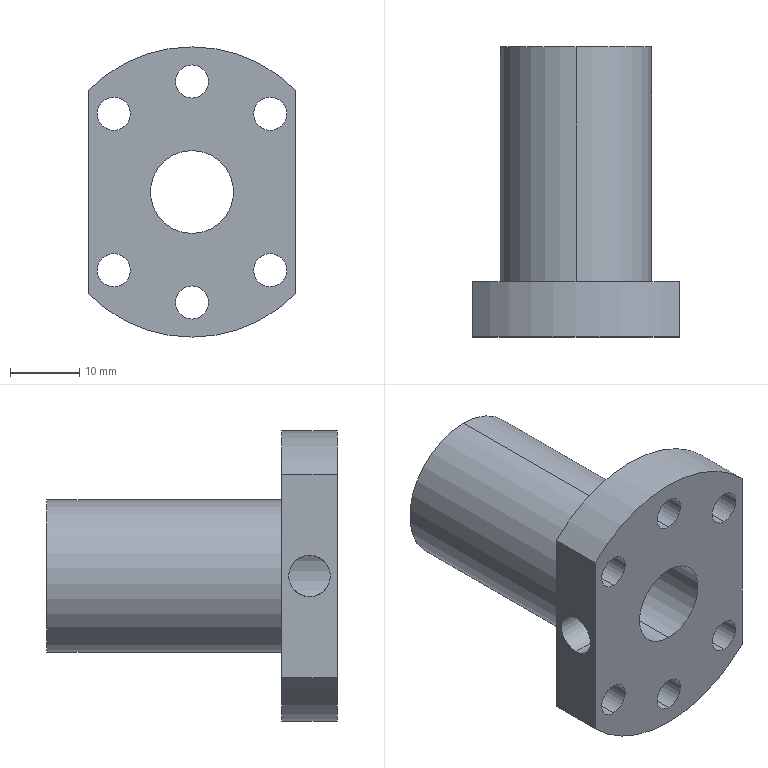Part | SolidWorks | features BaseBody 1 | 1 solid | 26 faces | box 30 x 42 x 42 mm | volume 16187 mm3 | cylinder 21 | plane 5 | commonest cylinder face diameters 4.8 x12 42 x3 6 x2 12 x2 22 x2
STEP:
#1=CARTESIAN_POINT('',(0.,42.,-11.));
#2=VERTEX_POINT('',#1);
#3=CARTESIAN_POINT('',(0.,42.,11.));
#4=VERTEX_POINT('',#3);
#5=CARTESIAN_POINT('',(0.,42.,0.));
#6=DIRECTION('',(0.,-1.,0.));
#7=DIRECTION('',(0.,0.,-1.));
#8=AXIS2_PLACEMENT_3D('',#5,#6,#7);
#9=CIRCLE('',#8,11.);
#10=EDGE_CURVE('',#2,#4,#9,.T.);
#11=ORIENTED_EDGE('',*,*,#10,.T.);
#12=CARTESIAN_POINT('',(0.,8.,11.));
#13=VERTEX_POINT('',#12);
#14=CARTESIAN_POINT('',(0.,42.,11.));
#15=DIRECTION('',(0.,-1.,0.));
#16=VECTOR('',#15,1000.);
#17=LINE('',#14,#16);
#18=EDGE_CURVE('',#4,#13,#17,.T.);
#19=ORIENTED_EDGE('',*,*,#18,.T.);
#20=CARTESIAN_POINT('',(0.,8.,-11.));
#21=VERTEX_POINT('',#20);
#22=CARTESIAN_POINT('',(0.,8.,0.));
#23=DIRECTION('',(0.,1.,0.));
#24=DIRECTION('',(0.,0.,-1.));
#25=AXIS2_PLACEMENT_3D('',#22,#23,#24);
#26=CIRCLE('',#25,11.);
#27=EDGE_CURVE('',#13,#21,#26,.T.);
#28=ORIENTED_EDGE('',*,*,#27,.T.);
#29=CARTESIAN_POINT('',(0.,42.,-11.));
#30=DIRECTION('',(0.,-1.,0.));
#31=VECTOR('',#30,1000.);
#32=LINE('',#29,#31);
#33=EDGE_CURVE('',#2,#21,#32,.T.);
#34=ORIENTED_EDGE('',*,*,#33,.F.);
#35=EDGE_LOOP('',(#11,#19,#28,#34));
#36=FACE_OUTER_BOUND('',#35,.T.);
#37=CARTESIAN_POINT('',(0.,42.,0.));
#38=DIRECTION('',(0.,-1.,0.));
#39=DIRECTION('',(0.,0.,-1.));
#40=AXIS2_PLACEMENT_3D('',#37,#38,#39);
#41=CYLINDRICAL_SURFACE('',#40,11.);
#42=ADVANCED_FACE('',(#36),#41,.T.);
#43=CARTESIAN_POINT('',(-11.314,8.,-8.914));
#44=VERTEX_POINT('',#43);
#45=CARTESIAN_POINT('',(-11.314,8.,-13.714));
#46=VERTEX_POINT('',#45);
#47=CARTESIAN_POINT('',(-11.314,8.,-11.314));
#48=DIRECTION('',(0.,-1.,0.));
#49=DIRECTION('',(0.,0.,-1.));
#50=AXIS2_PLACEMENT_3D('',#47,#48,#49);
#51=CIRCLE('',#50,2.4);
#52=EDGE_CURVE('',#44,#46,#51,.T.);
#53=ORIENTED_EDGE('',*,*,#52,.F.);
#54=CARTESIAN_POINT('',(-11.314,0.,-8.914));
#55=VERTEX_POINT('',#54);
#56=CARTESIAN_POINT('',(-11.314,8.,-8.914));
#57=DIRECTION('',(0.,-1.,0.));
#58=VECTOR('',#57,1000.);
#59=LINE('',#56,#58);
#60=EDGE_CURVE('',#44,#55,#59,.T.);
#61=ORIENTED_EDGE('',*,*,#60,.T.);
#62=CARTESIAN_POINT('',(-11.314,0.,-13.714));
#63=VERTEX_POINT('',#62);
#64=CARTESIAN_POINT('',(-11.314,0.,-11.314));
#65=DIRECTION('',(0.,1.,0.));
#66=DIRECTION('',(0.,0.,-1.));
#67=AXIS2_PLACEMENT_3D('',#64,#65,#66);
#68=CIRCLE('',#67,2.4);
#69=EDGE_CURVE('',#63,#55,#68,.T.);
#70=ORIENTED_EDGE('',*,*,#69,.F.);
#71=CARTESIAN_POINT('',(-11.314,8.,-13.714));
#72=DIRECTION('',(0.,-1.,0.));
#73=VECTOR('',#72,1000.);
#74=LINE('',#71,#73);
#75=EDGE_CURVE('',#46,#63,#74,.T.);
#76=ORIENTED_EDGE('',*,*,#75,.F.);
#77=EDGE_LOOP('',(#53,#61,#70,#76));
#78=FACE_OUTER_BOUND('',#77,.T.);
#79=CARTESIAN_POINT('',(-11.314,8.,-11.314));
#80=DIRECTION('',(0.,-1.,0.));
#81=DIRECTION('',(0.,0.,-1.));
#82=AXIS2_PLACEMENT_3D('',#79,#80,#81);
#83=CYLINDRICAL_SURFACE('',#82,2.4);
#84=ADVANCED_FACE('',(#78),#83,.F.);
#85=CARTESIAN_POINT('',(11.314,8.,13.714));
#86=VERTEX_POINT('',#85);
#87=CARTESIAN_POINT('',(11.314,8.,8.914));
#88=VERTEX_POINT('',#87);
#89=CARTESIAN_POINT('',(11.314,8.,11.314));
#90=DIRECTION('',(0.,-1.,0.));
#91=DIRECTION('',(0.,0.,-1.));
#92=AXIS2_PLACEMENT_3D('',#89,#90,#91);
#93=CIRCLE('',#92,2.4);
#94=EDGE_CURVE('',#86,#88,#93,.T.);
#95=ORIENTED_EDGE('',*,*,#94,.F.);
#96=CARTESIAN_POINT('',(11.314,0.,13.714));
#97=VERTEX_POINT('',#96);
#98=CARTESIAN_POINT('',(11.314,8.,13.714));
#99=DIRECTION('',(0.,-1.,0.));
#100=VECTOR('',#99,1000.);
#101=LINE('',#98,#100);
#102=EDGE_CURVE('',#86,#97,#101,.T.);
#103=ORIENTED_EDGE('',*,*,#102,.T.);
#104=CARTESIAN_POINT('',(11.314,0.,8.914));
#105=VERTEX_POINT('',#104);
#106=CARTESIAN_POINT('',(11.314,0.,11.314));
#107=DIRECTION('',(0.,1.,0.));
#108=DIRECTION('',(0.,0.,-1.));
#109=AXIS2_PLACEMENT_3D('',#106,#107,#108);
#110=CIRCLE('',#109,2.4);
#111=EDGE_CURVE('',#105,#97,#110,.T.);
#112=ORIENTED_EDGE('',*,*,#111,.F.);
#113=CARTESIAN_POINT('',(11.314,8.,8.914));
#114=DIRECTION('',(0.,-1.,0.));
#115=VECTOR('',#114,1000.);
#116=LINE('',#113,#115);
#117=EDGE_CURVE('',#88,#105,#116,.T.);
#118=ORIENTED_EDGE('',*,*,#117,.F.);
#119=EDGE_LOOP('',(#95,#103,#112,#118));
#120=FACE_OUTER_BOUND('',#119,.T.);
#121=CARTESIAN_POINT('',(11.314,8.,11.314));
#122=DIRECTION('',(0.,-1.,0.));
#123=DIRECTION('',(0.,0.,-1.));
#124=AXIS2_PLACEMENT_3D('',#121,#122,#123);
#125=CYLINDRICAL_SURFACE('',#124,2.4);
#126=ADVANCED_FACE('',(#120),#125,.F.);
#127=CARTESIAN_POINT('',(-11.314,8.,13.714));
#128=VERTEX_POINT('',#127);
#129=CARTESIAN_POINT('',(-11.314,8.,8.914));
#130=VERTEX_POINT('',#129);
#131=CARTESIAN_POINT('',(-11.314,8.,11.314));
#132=DIRECTION('',(0.,-1.,0.));
#133=DIRECTION('',(0.,0.,-1.));
#134=AXIS2_PLACEMENT_3D('',#131,#132,#133);
#135=CIRCLE('',#134,2.4);
#136=EDGE_CURVE('',#128,#130,#135,.T.);
#137=ORIENTED_EDGE('',*,*,#136,.F.);
#138=CARTESIAN_POINT('',(-11.314,0.,13.714));
#139=VERTEX_POINT('',#138);
#140=CARTESIAN_POINT('',(-11.314,8.,13.714));
#141=DIRECTION('',(0.,-1.,0.));
#142=VECTOR('',#141,1000.);
#143=LINE('',#140,#142);
#144=EDGE_CURVE('',#128,#139,#143,.T.);
#145=ORIENTED_EDGE('',*,*,#144,.T.);
#146=CARTESIAN_POINT('',(-11.314,0.,8.914));
#147=VERTEX_POINT('',#146);
#148=CARTESIAN_POINT('',(-11.314,0.,11.314));
#149=DIRECTION('',(0.,1.,0.));
#150=DIRECTION('',(0.,0.,-1.));
#151=AXIS2_PLACEMENT_3D('',#148,#149,#150);
#152=CIRCLE('',#151,2.4);
#153=EDGE_CURVE('',#147,#139,#152,.T.);
#154=ORIENTED_EDGE('',*,*,#153,.F.);
#155=CARTESIAN_POINT('',(-11.314,8.,8.914));
#156=DIRECTION('',(0.,-1.,0.));
#157=VECTOR('',#156,1000.);
#158=LINE('',#155,#157);
#159=EDGE_CURVE('',#130,#147,#158,.T.);
#160=ORIENTED_EDGE('',*,*,#159,.F.);
#161=EDGE_LOOP('',(#137,#145,#154,#160));
#162=FACE_OUTER_BOUND('',#161,.T.);
#163=CARTESIAN_POINT('',(-11.314,8.,11.314));
#164=DIRECTION('',(0.,-1.,0.));
#165=DIRECTION('',(0.,0.,-1.));
#166=AXIS2_PLACEMENT_3D('',#163,#164,#165);
#167=CYLINDRICAL_SURFACE('',#166,2.4);
#168=ADVANCED_FACE('',(#162),#167,.F.);
#169=CARTESIAN_POINT('',(0.,8.,18.4));
#170=VERTEX_POINT('',#169);
#171=CARTESIAN_POINT('',(0.,8.,13.6));
#172=VERTEX_POINT('',#171);
#173=CARTESIAN_POINT('',(0.,8.,16.));
#174=DIRECTION('',(0.,-1.,0.));
#175=DIRECTION('',(0.,0.,-1.));
#176=AXIS2_PLACEMENT_3D('',#173,#174,#175);
#177=CIRCLE('',#176,2.4);
#178=EDGE_CURVE('',#170,#172,#177,.T.);
#179=ORIENTED_EDGE('',*,*,#178,.F.);
#180=CARTESIAN_POINT('',(0.,0.,18.4));
#181=VERTEX_POINT('',#180);
#182=CARTESIAN_POINT('',(0.,8.,18.4));
#183=DIRECTION('',(0.,-1.,0.));
#184=VECTOR('',#183,1000.);
#185=LINE('',#182,#184);
#186=EDGE_CURVE('',#170,#181,#185,.T.);
#187=ORIENTED_EDGE('',*,*,#186,.T.);
#188=CARTESIAN_POINT('',(0.,0.,13.6));
#189=VERTEX_POINT('',#188);
#190=CARTESIAN_POINT('',(0.,0.,16.));
#191=DIRECTION('',(0.,1.,0.));
#192=DIRECTION('',(0.,0.,-1.));
#193=AXIS2_PLACEMENT_3D('',#190,#191,#192);
#194=CIRCLE('',#193,2.4);
#195=EDGE_CURVE('',#189,#181,#194,.T.);
#196=ORIENTED_EDGE('',*,*,#195,.F.);
#197=CARTESIAN_POINT('',(0.,8.,13.6));
#198=DIRECTION('',(0.,-1.,0.));
#199=VECTOR('',#198,1000.);
#200=LINE('',#197,#199);
#201=EDGE_CURVE('',#172,#189,#200,.T.);
#202=ORIENTED_EDGE('',*,*,#201,.F.);
#203=EDGE_LOOP('',(#179,#187,#196,#202));
#204=FACE_OUTER_BOUND('',#203,.T.);
#205=CARTESIAN_POINT('',(0.,8.,16.));
#206=DIRECTION('',(0.,-1.,0.));
#207=DIRECTION('',(0.,0.,-1.));
#208=AXIS2_PLACEMENT_3D('',#205,#206,#207);
#209=CYLINDRICAL_SURFACE('',#208,2.4);
#210=ADVANCED_FACE('',(#204),#209,.F.);
#211=CARTESIAN_POINT('',(0.,8.,-21.));
#212=VERTEX_POINT('',#211);
#213=CARTESIAN_POINT('',(-15.,8.,-14.697));
#214=VERTEX_POINT('',#213);
#215=CARTESIAN_POINT('',(0.,8.,0.));
#216=DIRECTION('',(0.,1.,0.));
#217=DIRECTION('',(0.,0.,-1.));
#218=AXIS2_PLACEMENT_3D('',#215,#216,#217);
#219=CIRCLE('',#218,21.);
#220=EDGE_CURVE('',#212,#214,#219,.T.);
#221=ORIENTED_EDGE('',*,*,#220,.F.);
#222=CARTESIAN_POINT('',(0.,0.,-21.));
#223=VERTEX_POINT('',#222);
#224=CARTESIAN_POINT('',(0.,8.,-21.));
#225=DIRECTION('',(0.,-1.,0.));
#226=VECTOR('',#225,1000.);
#227=LINE('',#224,#226);
#228=EDGE_CURVE('',#212,#223,#227,.T.);
#229=ORIENTED_EDGE('',*,*,#228,.T.);
#230=CARTESIAN_POINT('',(-15.,0.,-14.697));
#231=VERTEX_POINT('',#230);
#232=CARTESIAN_POINT('',(0.,0.,0.));
#233=DIRECTION('',(0.,1.,0.));
#234=DIRECTION('',(0.,0.,-1.));
#235=AXIS2_PLACEMENT_3D('',#232,#233,#234);
#236=CIRCLE('',#235,21.);
#237=EDGE_CURVE('',#223,#231,#236,.T.);
#238=ORIENTED_EDGE('',*,*,#237,.T.);
#239=CARTESIAN_POINT('',(-15.,8.,-14.697));
#240=DIRECTION('',(0.,1.,0.));
#241=VECTOR('',#240,1000.);
#242=LINE('',#239,#241);
#243=EDGE_CURVE('',#231,#214,#242,.T.);
#244=ORIENTED_EDGE('',*,*,#243,.T.);
#245=EDGE_LOOP('',(#221,#229,#238,#244));
#246=FACE_OUTER_BOUND('',#245,.T.);
#247=CARTESIAN_POINT('',(0.,8.,0.));
#248=DIRECTION('',(0.,-1.,0.));
#249=DIRECTION('',(0.,0.,-1.));
#250=AXIS2_PLACEMENT_3D('',#247,#248,#249);
#251=CYLINDRICAL_SURFACE('',#250,21.);
#252=ADVANCED_FACE('',(#246),#251,.T.);
#253=CARTESIAN_POINT('',(11.314,8.,-8.914));
#254=VERTEX_POINT('',#253);
#255=CARTESIAN_POINT('',(11.314,8.,-13.714));
#256=VERTEX_POINT('',#255);
#257=CARTESIAN_POINT('',(11.314,8.,-11.314));
#258=DIRECTION('',(0.,-1.,0.));
#259=DIRECTION('',(0.,0.,-1.));
#260=AXIS2_PLACEMENT_3D('',#257,#258,#259);
#261=CIRCLE('',#260,2.4);
#262=EDGE_CURVE('',#254,#256,#261,.T.);
#263=ORIENTED_EDGE('',*,*,#262,.F.);
#264=CARTESIAN_POINT('',(11.314,0.,-8.914));
#265=VERTEX_POINT('',#264);
#266=CARTESIAN_POINT('',(11.314,8.,-8.914));
#267=DIRECTION('',(0.,-1.,0.));
#268=VECTOR('',#267,1000.);
#269=LINE('',#266,#268);
#270=EDGE_CURVE('',#254,#265,#269,.T.);
#271=ORIENTED_EDGE('',*,*,#270,.T.);
#272=CARTESIAN_POINT('',(11.314,0.,-13.714));
#273=VERTEX_POINT('',#272);
#274=CARTESIAN_POINT('',(11.314,0.,-11.314));
#275=DIRECTION('',(0.,1.,0.));
#276=DIRECTION('',(0.,0.,-1.));
#277=AXIS2_PLACEMENT_3D('',#274,#275,#276);
#278=CIRCLE('',#277,2.4);
#279=EDGE_CURVE('',#273,#265,#278,.T.);
#280=ORIENTED_EDGE('',*,*,#279,.F.);
#281=CARTESIAN_POINT('',(11.314,8.,-13.714));
#282=DIRECTION('',(0.,-1.,0.));
#283=VECTOR('',#282,1000.);
#284=LINE('',#281,#283);
#285=EDGE_CURVE('',#256,#273,#284,.T.);
#286=ORIENTED_EDGE('',*,*,#285,.F.);
#287=EDGE_LOOP('',(#263,#271,#280,#286));
#288=FACE_OUTER_BOUND('',#287,.T.);
#289=CARTESIAN_POINT('',(11.314,8.,-11.314));
#290=DIRECTION('',(0.,-1.,0.));
#291=DIRECTION('',(0.,0.,-1.));
#292=AXIS2_PLACEMENT_3D('',#289,#290,#291);
#293=CYLINDRICAL_SURFACE('',#292,2.4);
#294=ADVANCED_FACE('',(#288),#293,.F.);
#295=CARTESIAN_POINT('',(0.,8.,-13.6));
#296=VERTEX_POINT('',#295);
#297=CARTESIAN_POINT('',(0.,8.,-18.4));
#298=VERTEX_POINT('',#297);
#299=CARTESIAN_POINT('',(0.,8.,-16.));
#300=DIRECTION('',(0.,-1.,0.));
#301=DIRECTION('',(0.,0.,-1.));
#302=AXIS2_PLACEMENT_3D('',#299,#300,#301);
#303=CIRCLE('',#302,2.4);
#304=EDGE_CURVE('',#296,#298,#303,.T.);
#305=ORIENTED_EDGE('',*,*,#304,.F.);
#306=CARTESIAN_POINT('',(0.,0.,-13.6));
#307=VERTEX_POINT('',#306);
#308=CARTESIAN_POINT('',(0.,8.,-13.6));
#309=DIRECTION('',(0.,-1.,0.));
#310=VECTOR('',#309,1000.);
#311=LINE('',#308,#310);
#312=EDGE_CURVE('',#296,#307,#311,.T.);
#313=ORIENTED_EDGE('',*,*,#312,.T.);
#314=CARTESIAN_POINT('',(0.,0.,-18.4));
#315=VERTEX_POINT('',#314);
#316=CARTESIAN_POINT('',(0.,0.,-16.));
#317=DIRECTION('',(0.,1.,0.));
#318=DIRECTION('',(0.,0.,-1.));
#319=AXIS2_PLACEMENT_3D('',#316,#317,#318);
#320=CIRCLE('',#319,2.4);
#321=EDGE_CURVE('',#315,#307,#320,.T.);
#322=ORIENTED_EDGE('',*,*,#321,.F.);
#323=CARTESIAN_POINT('',(0.,8.,-18.4));
#324=DIRECTION('',(0.,-1.,0.));
#325=VECTOR('',#324,1000.);
#326=LINE('',#323,#325);
#327=EDGE_CURVE('',#298,#315,#326,.T.);
#328=ORIENTED_EDGE('',*,*,#327,.F.);
#329=EDGE_LOOP('',(#305,#313,#322,#328));
#330=FACE_OUTER_BOUND('',#329,.T.);
#331=CARTESIAN_POINT('',(0.,8.,-16.));
#332=DIRECTION('',(0.,-1.,0.));
#333=DIRECTION('',(0.,0.,-1.));
#334=AXIS2_PLACEMENT_3D('',#331,#332,#333);
#335=CYLINDRICAL_SURFACE('',#334,2.4);
#336=ADVANCED_FACE('',(#330),#335,.F.);
#337=CARTESIAN_POINT('',(-5.196,4.,3.));
#338=VERTEX_POINT('',#337);
#339=CARTESIAN_POINT('',(-5.196,4.,-3.));
#340=VERTEX_POINT('',#339);
#341=CARTESIAN_POINT('',(-5.196,4.,3.));
#342=CARTESIAN_POINT('',(-5.196,3.798,3.));
#343=CARTESIAN_POINT('',(-5.208,3.6,2.98));
#344=CARTESIAN_POINT('',(-5.252,3.213,2.902));
#345=CARTESIAN_POINT('',(-5.285,3.021,2.843));
#346=CARTESIAN_POINT('',(-5.363,2.66,2.691));
#347=CARTESIAN_POINT('',(-5.409,2.489,2.599));
#348=CARTESIAN_POINT('',(-5.508,2.166,2.382));
#349=CARTESIAN_POINT('',(-5.56,2.016,2.259));
#350=CARTESIAN_POINT('',(-5.663,1.744,1.987));
#351=CARTESIAN_POINT('',(-5.714,1.62,1.837));
#352=CARTESIAN_POINT('',(-5.808,1.403,1.514));
#353=CARTESIAN_POINT('',(-5.851,1.31,1.343));
#354=CARTESIAN_POINT('',(-5.922,1.159,0.9829));
#355=CARTESIAN_POINT('',(-5.951,1.099,0.7906));
#356=CARTESIAN_POINT('',(-5.99,1.02,0.4015));
#357=CARTESIAN_POINT('',(-6.,1.,0.2044));
#358=CARTESIAN_POINT('',(-6.,0.9997,-0.1952));
#359=CARTESIAN_POINT('',(-5.99,1.02,-0.3971));
#360=CARTESIAN_POINT('',(-5.952,1.098,-0.7856));
#361=CARTESIAN_POINT('',(-5.923,1.156,-0.9764));
#362=CARTESIAN_POINT('',(-5.851,1.309,-1.341));
#363=CARTESIAN_POINT('',(-5.809,1.402,-1.512));
#364=CARTESIAN_POINT('',(-5.715,1.618,-1.835));
#365=CARTESIAN_POINT('',(-5.664,1.743,-1.986));
#366=CARTESIAN_POINT('',(-5.561,2.016,-2.258));
#367=CARTESIAN_POINT('',(-5.509,2.164,-2.381));
#368=CARTESIAN_POINT('',(-5.41,2.488,-2.598));
#369=CARTESIAN_POINT('',(-5.364,2.659,-2.691));
#370=CARTESIAN_POINT('',(-5.285,3.018,-2.841));
#371=CARTESIAN_POINT('',(-5.253,3.207,-2.9));
#372=CARTESIAN_POINT('',(-5.208,3.599,-2.98));
#373=CARTESIAN_POINT('',(-5.196,3.798,-3.));
#374=CARTESIAN_POINT('',(-5.196,4.,-3.));
#375=B_SPLINE_CURVE_WITH_KNOTS('',3,(#341,#342,#343,#344,#345,#346,#347,#348,#349,#350,#351,#352,#353,#354,#355,#356,#357,#358,#359,#360,#361,#362,#363,#364,#365,#366,#367,#368,#369,#370,#371,#372,#373,#374),.UNSPECIFIED.,.F.,.F.,(4,2,2,2,2,2,2,2,2,2,2,2,2,2,2,2,4),(0.,0.000596,0.001192,0.001788,0.002384,0.00298,0.003576,0.004172,0.004768,0.005364,0.00596,0.006556,0.007152,0.007748,0.008344,0.00894,0.009537),.UNSPECIFIED.);
#376=EDGE_CURVE('',#338,#340,#375,.T.);
#377=ORIENTED_EDGE('',*,*,#376,.F.);
#378=CARTESIAN_POINT('',(-5.196,4.,-3.));
#379=CARTESIAN_POINT('',(-5.196,4.202,-3.));
#380=CARTESIAN_POINT('',(-5.208,4.4,-2.98));
#381=CARTESIAN_POINT('',(-5.252,4.787,-2.902));
#382=CARTESIAN_POINT('',(-5.285,4.979,-2.843));
#383=CARTESIAN_POINT('',(-5.363,5.34,-2.691));
#384=CARTESIAN_POINT('',(-5.409,5.511,-2.599));
#385=CARTESIAN_POINT('',(-5.508,5.834,-2.382));
#386=CARTESIAN_POINT('',(-5.56,5.984,-2.259));
#387=CARTESIAN_POINT('',(-5.663,6.256,-1.987));
#388=CARTESIAN_POINT('',(-5.714,6.38,-1.837));
#389=CARTESIAN_POINT('',(-5.808,6.597,-1.514));
#390=CARTESIAN_POINT('',(-5.851,6.69,-1.343));
#391=CARTESIAN_POINT('',(-5.922,6.841,-0.9829));
#392=CARTESIAN_POINT('',(-5.951,6.901,-0.7906));
#393=CARTESIAN_POINT('',(-5.99,6.98,-0.4015));
#394=CARTESIAN_POINT('',(-6.,7.,-0.2044));
#395=CARTESIAN_POINT('',(-6.,7.,0.1952));
#396=CARTESIAN_POINT('',(-5.99,6.98,0.3971));
#397=CARTESIAN_POINT('',(-5.952,6.902,0.7856));
#398=CARTESIAN_POINT('',(-5.923,6.844,0.9764));
#399=CARTESIAN_POINT('',(-5.851,6.691,1.341));
#400=CARTESIAN_POINT('',(-5.809,6.598,1.512));
#401=CARTESIAN_POINT('',(-5.715,6.382,1.835));
#402=CARTESIAN_POINT('',(-5.664,6.257,1.986));
#403=CARTESIAN_POINT('',(-5.561,5.984,2.258));
#404=CARTESIAN_POINT('',(-5.509,5.836,2.381));
#405=CARTESIAN_POINT('',(-5.41,5.512,2.598));
#406=CARTESIAN_POINT('',(-5.364,5.341,2.691));
#407=CARTESIAN_POINT('',(-5.285,4.982,2.841));
#408=CARTESIAN_POINT('',(-5.253,4.793,2.9));
#409=CARTESIAN_POINT('',(-5.208,4.401,2.98));
#410=CARTESIAN_POINT('',(-5.196,4.202,3.));
#411=CARTESIAN_POINT('',(-5.196,4.,3.));
#412=B_SPLINE_CURVE_WITH_KNOTS('',3,(#378,#379,#380,#381,#382,#383,#384,#385,#386,#387,#388,#389,#390,#391,#392,#393,#394,#395,#396,#397,#398,#399,#400,#401,#402,#403,#404,#405,#406,#407,#408,#409,#410,#411),.UNSPECIFIED.,.F.,.F.,(4,2,2,2,2,2,2,2,2,2,2,2,2,2,2,2,4),(0.009537,0.01013,0.01073,0.01132,0.01192,0.01251,0.01311,0.01371,0.0143,0.0149,0.01549,0.01609,0.01668,0.01728,0.01788,0.01847,0.01907),.UNSPECIFIED.);
#413=EDGE_CURVE('',#340,#338,#412,.T.);
#414=ORIENTED_EDGE('',*,*,#413,.F.);
#415=EDGE_LOOP('',(#377,#414));
#416=FACE_BOUND('',#415,.T.);
#417=CARTESIAN_POINT('',(0.,42.,6.));
#418=VERTEX_POINT('',#417);
#419=CARTESIAN_POINT('',(0.,42.,-6.));
#420=VERTEX_POINT('',#419);
#421=CARTESIAN_POINT('',(0.,42.,0.));
#422=DIRECTION('',(0.,-1.,0.));
#423=DIRECTION('',(0.,0.,-1.));
#424=AXIS2_PLACEMENT_3D('',#421,#422,#423);
#425=CIRCLE('',#424,6.);
#426=EDGE_CURVE('',#418,#420,#425,.T.);
#427=ORIENTED_EDGE('',*,*,#426,.F.);
#428=CARTESIAN_POINT('',(0.,0.,6.));
#429=VERTEX_POINT('',#428);
#430=CARTESIAN_POINT('',(0.,42.,6.));
#431=DIRECTION('',(0.,-1.,0.));
#432=VECTOR('',#431,1000.);
#433=LINE('',#430,#432);
#434=EDGE_CURVE('',#418,#429,#433,.T.);
#435=ORIENTED_EDGE('',*,*,#434,.T.);
#436=CARTESIAN_POINT('',(0.,0.,-6.));
#437=VERTEX_POINT('',#436);
#438=CARTESIAN_POINT('',(0.,0.,0.));
#439=DIRECTION('',(0.,1.,0.));
#440=DIRECTION('',(0.,0.,-1.));
#441=AXIS2_PLACEMENT_3D('',#438,#439,#440);
#442=CIRCLE('',#441,6.);
#443=EDGE_CURVE('',#437,#429,#442,.T.);
#444=ORIENTED_EDGE('',*,*,#443,.F.);
#445=CARTESIAN_POINT('',(0.,42.,-6.));
#446=DIRECTION('',(0.,-1.,0.));
#447=VECTOR('',#446,1000.);
#448=LINE('',#445,#447);
#449=EDGE_CURVE('',#420,#437,#448,.T.);
#450=ORIENTED_EDGE('',*,*,#449,.F.);
#451=EDGE_LOOP('',(#427,#435,#444,#450));
#452=FACE_OUTER_BOUND('',#451,.T.);
#453=CARTESIAN_POINT('',(0.,42.,0.));
#454=DIRECTION('',(0.,-1.,0.));
#455=DIRECTION('',(0.,0.,-1.));
#456=AXIS2_PLACEMENT_3D('',#453,#454,#455);
#457=CYLINDRICAL_SURFACE('',#456,6.);
#458=ADVANCED_FACE('',(#416,#452),#457,.F.);
#459=ORIENTED_EDGE('',*,*,#376,.T.);
#460=CARTESIAN_POINT('',(-15.,4.,-3.));
#461=VERTEX_POINT('',#460);
#462=CARTESIAN_POINT('',(5.,4.,-3.));
#463=DIRECTION('',(-1.,0.,0.));
#464=VECTOR('',#463,1000.);
#465=LINE('',#462,#464);
#466=EDGE_CURVE('',#340,#461,#465,.T.);
#467=ORIENTED_EDGE('',*,*,#466,.T.);
#468=CARTESIAN_POINT('',(-15.,4.,3.));
#469=VERTEX_POINT('',#468);
#470=CARTESIAN_POINT('',(-15.,4.,0.));
#471=DIRECTION('',(-1.,0.,0.));
#472=DIRECTION('',(0.,0.,1.));
#473=AXIS2_PLACEMENT_3D('',#470,#471,#472);
#474=CIRCLE('',#473,3.);
#475=EDGE_CURVE('',#461,#469,#474,.T.);
#476=ORIENTED_EDGE('',*,*,#475,.T.);
#477=CARTESIAN_POINT('',(5.,4.,3.));
#478=DIRECTION('',(-1.,0.,0.));
#479=VECTOR('',#478,1000.);
#480=LINE('',#477,#479);
#481=EDGE_CURVE('',#338,#469,#480,.T.);
#482=ORIENTED_EDGE('',*,*,#481,.F.);
#483=EDGE_LOOP('',(#459,#467,#476,#482));
#484=FACE_OUTER_BOUND('',#483,.T.);
#485=CARTESIAN_POINT('',(5.,4.,0.));
#486=DIRECTION('',(-1.,0.,0.));
#487=DIRECTION('',(0.,0.,1.));
#488=AXIS2_PLACEMENT_3D('',#485,#486,#487);
#489=CYLINDRICAL_SURFACE('',#488,3.);
#490=ADVANCED_FACE('',(#484),#489,.F.);
#491=ORIENTED_EDGE('',*,*,#18,.F.);
#492=CARTESIAN_POINT('',(0.,42.,0.));
#493=DIRECTION('',(0.,-1.,0.));
#494=DIRECTION('',(0.,0.,-1.));
#495=AXIS2_PLACEMENT_3D('',#492,#493,#494);
#496=CIRCLE('',#495,11.);
#497=EDGE_CURVE('',#4,#2,#496,.T.);
#498=ORIENTED_EDGE('',*,*,#497,.T.);
#499=ORIENTED_EDGE('',*,*,#33,.T.);
#500=CARTESIAN_POINT('',(0.,8.,0.));
#501=DIRECTION('',(0.,1.,0.));
#502=DIRECTION('',(0.,0.,-1.));
#503=AXIS2_PLACEMENT_3D('',#500,#501,#502);
#504=CIRCLE('',#503,11.);
#505=EDGE_CURVE('',#21,#13,#504,.T.);
#506=ORIENTED_EDGE('',*,*,#505,.T.);
#507=EDGE_LOOP('',(#491,#498,#499,#506));
#508=FACE_OUTER_BOUND('',#507,.T.);
#509=CARTESIAN_POINT('',(0.,42.,0.));
#510=DIRECTION('',(0.,-1.,0.));
#511=DIRECTION('',(0.,0.,-1.));
#512=AXIS2_PLACEMENT_3D('',#509,#510,#511);
#513=CYLINDRICAL_SURFACE('',#512,11.);
#514=ADVANCED_FACE('',(#508),#513,.T.);
#515=CARTESIAN_POINT('',(-11.314,8.,-11.314));
#516=DIRECTION('',(0.,-1.,0.));
#517=DIRECTION('',(0.,0.,-1.));
#518=AXIS2_PLACEMENT_3D('',#515,#516,#517);
#519=CIRCLE('',#518,2.4);
#520=EDGE_CURVE('',#46,#44,#519,.T.);
#521=ORIENTED_EDGE('',*,*,#520,.T.);
#522=ORIENTED_EDGE('',*,*,#52,.T.);
#523=EDGE_LOOP('',(#521,#522));
#524=FACE_BOUND('',#523,.T.);
#525=CARTESIAN_POINT('',(11.314,8.,11.314));
#526=DIRECTION('',(0.,-1.,0.));
#527=DIRECTION('',(0.,0.,-1.));
#528=AXIS2_PLACEMENT_3D('',#525,#526,#527);
#529=CIRCLE('',#528,2.4);
#530=EDGE_CURVE('',#88,#86,#529,.T.);
#531=ORIENTED_EDGE('',*,*,#530,.T.);
#532=ORIENTED_EDGE('',*,*,#94,.T.);
#533=EDGE_LOOP('',(#531,#532));
#534=FACE_BOUND('',#533,.T.);
#535=CARTESIAN_POINT('',(-11.314,8.,11.314));
#536=DIRECTION('',(0.,-1.,0.));
#537=DIRECTION('',(0.,0.,-1.));
#538=AXIS2_PLACEMENT_3D('',#535,#536,#537);
#539=CIRCLE('',#538,2.4);
#540=EDGE_CURVE('',#130,#128,#539,.T.);
#541=ORIENTED_EDGE('',*,*,#540,.T.);
#542=ORIENTED_EDGE('',*,*,#136,.T.);
#543=EDGE_LOOP('',(#541,#542));
#544=FACE_BOUND('',#543,.T.);
#545=CARTESIAN_POINT('',(0.,8.,16.));
#546=DIRECTION('',(0.,-1.,0.));
#547=DIRECTION('',(0.,0.,-1.));
#548=AXIS2_PLACEMENT_3D('',#545,#546,#547);
#549=CIRCLE('',#548,2.4);
#550=EDGE_CURVE('',#172,#170,#549,.T.);
#551=ORIENTED_EDGE('',*,*,#550,.T.);
#552=ORIENTED_EDGE('',*,*,#178,.T.);
#553=EDGE_LOOP('',(#551,#552));
#554=FACE_BOUND('',#553,.T.);
#555=ORIENTED_EDGE('',*,*,#505,.F.);
#556=ORIENTED_EDGE('',*,*,#27,.F.);
#557=EDGE_LOOP('',(#555,#556));
#558=FACE_BOUND('',#557,.T.);
#559=CARTESIAN_POINT('',(-15.,8.,14.697));
#560=VERTEX_POINT('',#559);
#561=CARTESIAN_POINT('',(-15.,8.,0.));
#562=DIRECTION('',(0.,0.,1.));
#563=VECTOR('',#562,1000.);
#564=LINE('',#561,#563);
#565=EDGE_CURVE('',#214,#560,#564,.T.);
#566=ORIENTED_EDGE('',*,*,#565,.T.);
#567=CARTESIAN_POINT('',(15.,8.,14.697));
#568=VERTEX_POINT('',#567);
#569=CARTESIAN_POINT('',(0.,8.,0.));
#570=DIRECTION('',(0.,1.,0.));
#571=DIRECTION('',(0.,0.,-1.));
#572=AXIS2_PLACEMENT_3D('',#569,#570,#571);
#573=CIRCLE('',#572,21.);
#574=EDGE_CURVE('',#560,#568,#573,.T.);
#575=ORIENTED_EDGE('',*,*,#574,.T.);
#576=CARTESIAN_POINT('',(15.,8.,-14.697));
#577=VERTEX_POINT('',#576);
#578=CARTESIAN_POINT('',(15.,8.,0.));
#579=DIRECTION('',(0.,0.,-1.));
#580=VECTOR('',#579,1000.);
#581=LINE('',#578,#580);
#582=EDGE_CURVE('',#568,#577,#581,.T.);
#583=ORIENTED_EDGE('',*,*,#582,.T.);
#584=CARTESIAN_POINT('',(0.,8.,0.));
#585=DIRECTION('',(0.,1.,0.));
#586=DIRECTION('',(0.,0.,-1.));
#587=AXIS2_PLACEMENT_3D('',#584,#585,#586);
#588=CIRCLE('',#587,21.);
#589=EDGE_CURVE('',#577,#212,#588,.T.);
#590=ORIENTED_EDGE('',*,*,#589,.T.);
#591=ORIENTED_EDGE('',*,*,#220,.T.);
#592=EDGE_LOOP('',(#566,#575,#583,#590,#591));
#593=FACE_OUTER_BOUND('',#592,.T.);
#594=CARTESIAN_POINT('',(11.314,8.,-11.314));
#595=DIRECTION('',(0.,-1.,0.));
#596=DIRECTION('',(0.,0.,-1.));
#597=AXIS2_PLACEMENT_3D('',#594,#595,#596);
#598=CIRCLE('',#597,2.4);
#599=EDGE_CURVE('',#256,#254,#598,.T.);
#600=ORIENTED_EDGE('',*,*,#599,.T.);
#601=ORIENTED_EDGE('',*,*,#262,.T.);
#602=EDGE_LOOP('',(#600,#601));
#603=FACE_BOUND('',#602,.T.);
#604=CARTESIAN_POINT('',(0.,8.,-16.));
#605=DIRECTION('',(0.,-1.,0.));
#606=DIRECTION('',(0.,0.,-1.));
#607=AXIS2_PLACEMENT_3D('',#604,#605,#606);
#608=CIRCLE('',#607,2.4);
#609=EDGE_CURVE('',#298,#296,#608,.T.);
#610=ORIENTED_EDGE('',*,*,#609,.T.);
#611=ORIENTED_EDGE('',*,*,#304,.T.);
#612=EDGE_LOOP('',(#610,#611));
#613=FACE_BOUND('',#612,.T.);
#614=CARTESIAN_POINT('',(0.,8.,0.));
#615=DIRECTION('',(0.,1.,0.));
#616=DIRECTION('',(0.,0.,1.));
#617=AXIS2_PLACEMENT_3D('',#614,#615,#616);
#618=PLANE('',#617);
#619=ADVANCED_FACE('',(#524,#534,#544,#554,#558,#593,#603,#613),#618,.T.);
#620=ORIENTED_EDGE('',*,*,#10,.F.);
#621=ORIENTED_EDGE('',*,*,#497,.F.);
#622=EDGE_LOOP('',(#620,#621));
#623=FACE_OUTER_BOUND('',#622,.T.);
#624=CARTESIAN_POINT('',(0.,42.,0.));
#625=DIRECTION('',(0.,-1.,0.));
#626=DIRECTION('',(0.,0.,-1.));
#627=AXIS2_PLACEMENT_3D('',#624,#625,#626);
#628=CIRCLE('',#627,6.);
#629=EDGE_CURVE('',#420,#418,#628,.T.);
#630=ORIENTED_EDGE('',*,*,#629,.T.);
#631=ORIENTED_EDGE('',*,*,#426,.T.);
#632=EDGE_LOOP('',(#630,#631));
#633=FACE_BOUND('',#632,.T.);
#634=CARTESIAN_POINT('',(0.,42.,0.));
#635=DIRECTION('',(0.,1.,0.));
#636=DIRECTION('',(0.,0.,1.));
#637=AXIS2_PLACEMENT_3D('',#634,#635,#636);
#638=PLANE('',#637);
#639=ADVANCED_FACE('',(#623,#633),#638,.T.);
#640=ORIENTED_EDGE('',*,*,#60,.F.);
#641=ORIENTED_EDGE('',*,*,#520,.F.);
#642=ORIENTED_EDGE('',*,*,#75,.T.);
#643=CARTESIAN_POINT('',(-11.314,0.,-11.314));
#644=DIRECTION('',(0.,1.,0.));
#645=DIRECTION('',(0.,0.,-1.));
#646=AXIS2_PLACEMENT_3D('',#643,#644,#645);
#647=CIRCLE('',#646,2.4);
#648=EDGE_CURVE('',#55,#63,#647,.T.);
#649=ORIENTED_EDGE('',*,*,#648,.F.);
#650=EDGE_LOOP('',(#640,#641,#642,#649));
#651=FACE_OUTER_BOUND('',#650,.T.);
#652=CARTESIAN_POINT('',(-11.314,8.,-11.314));
#653=DIRECTION('',(0.,-1.,0.));
#654=DIRECTION('',(0.,0.,-1.));
#655=AXIS2_PLACEMENT_3D('',#652,#653,#654);
#656=CYLINDRICAL_SURFACE('',#655,2.4);
#657=ADVANCED_FACE('',(#651),#656,.F.);
#658=ORIENTED_EDGE('',*,*,#102,.F.);
#659=ORIENTED_EDGE('',*,*,#530,.F.);
#660=ORIENTED_EDGE('',*,*,#117,.T.);
#661=CARTESIAN_POINT('',(11.314,0.,11.314));
#662=DIRECTION('',(0.,1.,0.));
#663=DIRECTION('',(0.,0.,-1.));
#664=AXIS2_PLACEMENT_3D('',#661,#662,#663);
#665=CIRCLE('',#664,2.4);
#666=EDGE_CURVE('',#97,#105,#665,.T.);
#667=ORIENTED_EDGE('',*,*,#666,.F.);
#668=EDGE_LOOP('',(#658,#659,#660,#667));
#669=FACE_OUTER_BOUND('',#668,.T.);
#670=CARTESIAN_POINT('',(11.314,8.,11.314));
#671=DIRECTION('',(0.,-1.,0.));
#672=DIRECTION('',(0.,0.,-1.));
#673=AXIS2_PLACEMENT_3D('',#670,#671,#672);
#674=CYLINDRICAL_SURFACE('',#673,2.4);
#675=ADVANCED_FACE('',(#669),#674,.F.);
#676=ORIENTED_EDGE('',*,*,#144,.F.);
#677=ORIENTED_EDGE('',*,*,#540,.F.);
#678=ORIENTED_EDGE('',*,*,#159,.T.);
#679=CARTESIAN_POINT('',(-11.314,0.,11.314));
#680=DIRECTION('',(0.,1.,0.));
#681=DIRECTION('',(0.,0.,-1.));
#682=AXIS2_PLACEMENT_3D('',#679,#680,#681);
#683=CIRCLE('',#682,2.4);
#684=EDGE_CURVE('',#139,#147,#683,.T.);
#685=ORIENTED_EDGE('',*,*,#684,.F.);
#686=EDGE_LOOP('',(#676,#677,#678,#685));
#687=FACE_OUTER_BOUND('',#686,.T.);
#688=CARTESIAN_POINT('',(-11.314,8.,11.314));
#689=DIRECTION('',(0.,-1.,0.));
#690=DIRECTION('',(0.,0.,-1.));
#691=AXIS2_PLACEMENT_3D('',#688,#689,#690);
#692=CYLINDRICAL_SURFACE('',#691,2.4);
#693=ADVANCED_FACE('',(#687),#692,.F.);
#694=ORIENTED_EDGE('',*,*,#186,.F.);
#695=ORIENTED_EDGE('',*,*,#550,.F.);
#696=ORIENTED_EDGE('',*,*,#201,.T.);
#697=CARTESIAN_POINT('',(0.,0.,16.));
#698=DIRECTION('',(0.,1.,0.));
#699=DIRECTION('',(0.,0.,-1.));
#700=AXIS2_PLACEMENT_3D('',#697,#698,#699);
#701=CIRCLE('',#700,2.4);
#702=EDGE_CURVE('',#181,#189,#701,.T.);
#703=ORIENTED_EDGE('',*,*,#702,.F.);
#704=EDGE_LOOP('',(#694,#695,#696,#703));
#705=FACE_OUTER_BOUND('',#704,.T.);
#706=CARTESIAN_POINT('',(0.,8.,16.));
#707=DIRECTION('',(0.,-1.,0.));
#708=DIRECTION('',(0.,0.,-1.));
#709=AXIS2_PLACEMENT_3D('',#706,#707,#708);
#710=CYLINDRICAL_SURFACE('',#709,2.4);
#711=ADVANCED_FACE('',(#705),#710,.F.);
#712=ORIENTED_EDGE('',*,*,#574,.F.);
#713=CARTESIAN_POINT('',(-15.,0.,14.697));
#714=VERTEX_POINT('',#713);
#715=CARTESIAN_POINT('',(-15.,8.,14.697));
#716=DIRECTION('',(0.,-1.,0.));
#717=VECTOR('',#716,1000.);
#718=LINE('',#715,#717);
#719=EDGE_CURVE('',#560,#714,#718,.T.);
#720=ORIENTED_EDGE('',*,*,#719,.T.);
#721=CARTESIAN_POINT('',(15.,0.,14.697));
#722=VERTEX_POINT('',#721);
#723=CARTESIAN_POINT('',(0.,0.,0.));
#724=DIRECTION('',(0.,1.,0.));
#725=DIRECTION('',(0.,0.,-1.));
#726=AXIS2_PLACEMENT_3D('',#723,#724,#725);
#727=CIRCLE('',#726,21.);
#728=EDGE_CURVE('',#714,#722,#727,.T.);
#729=ORIENTED_EDGE('',*,*,#728,.T.);
#730=CARTESIAN_POINT('',(15.,8.,14.697));
#731=DIRECTION('',(0.,1.,0.));
#732=VECTOR('',#731,1000.);
#733=LINE('',#730,#732);
#734=EDGE_CURVE('',#722,#568,#733,.T.);
#735=ORIENTED_EDGE('',*,*,#734,.T.);
#736=EDGE_LOOP('',(#712,#720,#729,#735));
#737=FACE_OUTER_BOUND('',#736,.T.);
#738=CARTESIAN_POINT('',(0.,8.,0.));
#739=DIRECTION('',(0.,-1.,0.));
#740=DIRECTION('',(0.,0.,-1.));
#741=AXIS2_PLACEMENT_3D('',#738,#739,#740);
#742=CYLINDRICAL_SURFACE('',#741,21.);
#743=ADVANCED_FACE('',(#737),#742,.T.);
#744=ORIENTED_EDGE('',*,*,#719,.F.);
#745=ORIENTED_EDGE('',*,*,#565,.F.);
#746=ORIENTED_EDGE('',*,*,#243,.F.);
#747=CARTESIAN_POINT('',(-15.,0.,0.));
#748=DIRECTION('',(0.,0.,-1.));
#749=VECTOR('',#748,1000.);
#750=LINE('',#747,#749);
#751=EDGE_CURVE('',#714,#231,#750,.T.);
#752=ORIENTED_EDGE('',*,*,#751,.F.);
#753=EDGE_LOOP('',(#744,#745,#746,#752));
#754=FACE_OUTER_BOUND('',#753,.T.);
#755=CARTESIAN_POINT('',(-15.,4.,0.));
#756=DIRECTION('',(-1.,0.,0.));
#757=DIRECTION('',(0.,0.,1.));
#758=AXIS2_PLACEMENT_3D('',#755,#756,#757);
#759=CIRCLE('',#758,3.);
#760=EDGE_CURVE('',#469,#461,#759,.T.);
#761=ORIENTED_EDGE('',*,*,#760,.F.);
#762=ORIENTED_EDGE('',*,*,#475,.F.);
#763=EDGE_LOOP('',(#761,#762));
#764=FACE_BOUND('',#763,.T.);
#765=CARTESIAN_POINT('',(-15.,8.,0.));
#766=DIRECTION('',(1.,0.,0.));
#767=DIRECTION('',(0.,0.,-1.));
#768=AXIS2_PLACEMENT_3D('',#765,#766,#767);
#769=PLANE('',#768);
#770=ADVANCED_FACE('',(#754,#764),#769,.F.);
#771=ORIENTED_EDGE('',*,*,#228,.F.);
#772=ORIENTED_EDGE('',*,*,#589,.F.);
#773=CARTESIAN_POINT('',(15.,0.,-14.697));
#774=VERTEX_POINT('',#773);
#775=CARTESIAN_POINT('',(15.,8.,-14.697));
#776=DIRECTION('',(0.,-1.,0.));
#777=VECTOR('',#776,1000.);
#778=LINE('',#775,#777);
#779=EDGE_CURVE('',#577,#774,#778,.T.);
#780=ORIENTED_EDGE('',*,*,#779,.T.);
#781=CARTESIAN_POINT('',(0.,0.,0.));
#782=DIRECTION('',(0.,1.,0.));
#783=DIRECTION('',(0.,0.,-1.));
#784=AXIS2_PLACEMENT_3D('',#781,#782,#783);
#785=CIRCLE('',#784,21.);
#786=EDGE_CURVE('',#774,#223,#785,.T.);
#787=ORIENTED_EDGE('',*,*,#786,.T.);
#788=EDGE_LOOP('',(#771,#772,#780,#787));
#789=FACE_OUTER_BOUND('',#788,.T.);
#790=CARTESIAN_POINT('',(0.,8.,0.));
#791=DIRECTION('',(0.,-1.,0.));
#792=DIRECTION('',(0.,0.,-1.));
#793=AXIS2_PLACEMENT_3D('',#790,#791,#792);
#794=CYLINDRICAL_SURFACE('',#793,21.);
#795=ADVANCED_FACE('',(#789),#794,.T.);
#796=ORIENTED_EDGE('',*,*,#582,.F.);
#797=ORIENTED_EDGE('',*,*,#734,.F.);
#798=CARTESIAN_POINT('',(15.,0.,0.));
#799=DIRECTION('',(0.,0.,-1.));
#800=VECTOR('',#799,1000.);
#801=LINE('',#798,#800);
#802=EDGE_CURVE('',#722,#774,#801,.T.);
#803=ORIENTED_EDGE('',*,*,#802,.T.);
#804=ORIENTED_EDGE('',*,*,#779,.F.);
#805=EDGE_LOOP('',(#796,#797,#803,#804));
#806=FACE_OUTER_BOUND('',#805,.T.);
#807=CARTESIAN_POINT('',(15.,8.,0.));
#808=DIRECTION('',(1.,0.,0.));
#809=DIRECTION('',(0.,0.,-1.));
#810=AXIS2_PLACEMENT_3D('',#807,#808,#809);
#811=PLANE('',#810);
#812=ADVANCED_FACE('',(#806),#811,.T.);
#813=ORIENTED_EDGE('',*,*,#270,.F.);
#814=ORIENTED_EDGE('',*,*,#599,.F.);
#815=ORIENTED_EDGE('',*,*,#285,.T.);
#816=CARTESIAN_POINT('',(11.314,0.,-11.314));
#817=DIRECTION('',(0.,1.,0.));
#818=DIRECTION('',(0.,0.,-1.));
#819=AXIS2_PLACEMENT_3D('',#816,#817,#818);
#820=CIRCLE('',#819,2.4);
#821=EDGE_CURVE('',#265,#273,#820,.T.);
#822=ORIENTED_EDGE('',*,*,#821,.F.);
#823=EDGE_LOOP('',(#813,#814,#815,#822));
#824=FACE_OUTER_BOUND('',#823,.T.);
#825=CARTESIAN_POINT('',(11.314,8.,-11.314));
#826=DIRECTION('',(0.,-1.,0.));
#827=DIRECTION('',(0.,0.,-1.));
#828=AXIS2_PLACEMENT_3D('',#825,#826,#827);
#829=CYLINDRICAL_SURFACE('',#828,2.4);
#830=ADVANCED_FACE('',(#824),#829,.F.);
#831=ORIENTED_EDGE('',*,*,#312,.F.);
#832=ORIENTED_EDGE('',*,*,#609,.F.);
#833=ORIENTED_EDGE('',*,*,#327,.T.);
#834=CARTESIAN_POINT('',(0.,0.,-16.));
#835=DIRECTION('',(0.,1.,0.));
#836=DIRECTION('',(0.,0.,-1.));
#837=AXIS2_PLACEMENT_3D('',#834,#835,#836);
#838=CIRCLE('',#837,2.4);
#839=EDGE_CURVE('',#307,#315,#838,.T.);
#840=ORIENTED_EDGE('',*,*,#839,.F.);
#841=EDGE_LOOP('',(#831,#832,#833,#840));
#842=FACE_OUTER_BOUND('',#841,.T.);
#843=CARTESIAN_POINT('',(0.,8.,-16.));
#844=DIRECTION('',(0.,-1.,0.));
#845=DIRECTION('',(0.,0.,-1.));
#846=AXIS2_PLACEMENT_3D('',#843,#844,#845);
#847=CYLINDRICAL_SURFACE('',#846,2.4);
#848=ADVANCED_FACE('',(#842),#847,.F.);
#849=ORIENTED_EDGE('',*,*,#434,.F.);
#850=ORIENTED_EDGE('',*,*,#629,.F.);
#851=ORIENTED_EDGE('',*,*,#449,.T.);
#852=CARTESIAN_POINT('',(0.,0.,0.));
#853=DIRECTION('',(0.,1.,0.));
#854=DIRECTION('',(0.,0.,-1.));
#855=AXIS2_PLACEMENT_3D('',#852,#853,#854);
#856=CIRCLE('',#855,6.);
#857=EDGE_CURVE('',#429,#437,#856,.T.);
#858=ORIENTED_EDGE('',*,*,#857,.F.);
#859=EDGE_LOOP('',(#849,#850,#851,#858));
#860=FACE_OUTER_BOUND('',#859,.T.);
#861=CARTESIAN_POINT('',(0.,42.,0.));
#862=DIRECTION('',(0.,-1.,0.));
#863=DIRECTION('',(0.,0.,-1.));
#864=AXIS2_PLACEMENT_3D('',#861,#862,#863);
#865=CYLINDRICAL_SURFACE('',#864,6.);
#866=ADVANCED_FACE('',(#860),#865,.F.);
#867=ORIENTED_EDGE('',*,*,#443,.T.);
#868=ORIENTED_EDGE('',*,*,#857,.T.);
#869=EDGE_LOOP('',(#867,#868));
#870=FACE_BOUND('',#869,.T.);
#871=ORIENTED_EDGE('',*,*,#69,.T.);
#872=ORIENTED_EDGE('',*,*,#648,.T.);
#873=EDGE_LOOP('',(#871,#872));
#874=FACE_BOUND('',#873,.T.);
#875=ORIENTED_EDGE('',*,*,#111,.T.);
#876=ORIENTED_EDGE('',*,*,#666,.T.);
#877=EDGE_LOOP('',(#875,#876));
#878=FACE_BOUND('',#877,.T.);
#879=ORIENTED_EDGE('',*,*,#153,.T.);
#880=ORIENTED_EDGE('',*,*,#684,.T.);
#881=EDGE_LOOP('',(#879,#880));
#882=FACE_BOUND('',#881,.T.);
#883=ORIENTED_EDGE('',*,*,#195,.T.);
#884=ORIENTED_EDGE('',*,*,#702,.T.);
#885=EDGE_LOOP('',(#883,#884));
#886=FACE_BOUND('',#885,.T.);
#887=ORIENTED_EDGE('',*,*,#728,.F.);
#888=ORIENTED_EDGE('',*,*,#751,.T.);
#889=ORIENTED_EDGE('',*,*,#237,.F.);
#890=ORIENTED_EDGE('',*,*,#786,.F.);
#891=ORIENTED_EDGE('',*,*,#802,.F.);
#892=EDGE_LOOP('',(#887,#888,#889,#890,#891));
#893=FACE_OUTER_BOUND('',#892,.T.);
#894=ORIENTED_EDGE('',*,*,#279,.T.);
#895=ORIENTED_EDGE('',*,*,#821,.T.);
#896=EDGE_LOOP('',(#894,#895));
#897=FACE_BOUND('',#896,.T.);
#898=ORIENTED_EDGE('',*,*,#321,.T.);
#899=ORIENTED_EDGE('',*,*,#839,.T.);
#900=EDGE_LOOP('',(#898,#899));
#901=FACE_BOUND('',#900,.T.);
#902=CARTESIAN_POINT('',(0.,0.,0.));
#903=DIRECTION('',(0.,1.,0.));
#904=DIRECTION('',(0.,0.,1.));
#905=AXIS2_PLACEMENT_3D('',#902,#903,#904);
#906=PLANE('',#905);
#907=ADVANCED_FACE('',(#870,#874,#878,#882,#886,#893,#897,#901),#906,.F.);
#908=ORIENTED_EDGE('',*,*,#466,.F.);
#909=ORIENTED_EDGE('',*,*,#413,.T.);
#910=ORIENTED_EDGE('',*,*,#481,.T.);
#911=ORIENTED_EDGE('',*,*,#760,.T.);
#912=EDGE_LOOP('',(#908,#909,#910,#911));
#913=FACE_OUTER_BOUND('',#912,.T.);
#914=CARTESIAN_POINT('',(5.,4.,0.));
#915=DIRECTION('',(-1.,0.,0.));
#916=DIRECTION('',(0.,0.,1.));
#917=AXIS2_PLACEMENT_3D('',#914,#915,#916);
#918=CYLINDRICAL_SURFACE('',#917,3.);
#919=ADVANCED_FACE('',(#913),#918,.F.);
#920=CLOSED_SHELL('',(#42,#84,#126,#168,#210,#252,#294,#336,#458,#490,#514,#619,#639,#657,#675,#693,#711,#743,#770,#795,#812,#830,#848,#866,#907,#919));
#921=MANIFOLD_SOLID_BREP('',#920);
#922=CARTESIAN_POINT('',(0.,0.,0.));
#923=DIRECTION('',(0.,0.,1.));
#924=DIRECTION('',(1.,0.,0.));
#925=AXIS2_PLACEMENT_3D('',#922,#923,#924);
#926=(LENGTH_UNIT()NAMED_UNIT(*)SI_UNIT(.MILLI.,.METRE.));
#927=UNCERTAINTY_MEASURE_WITH_UNIT(LENGTH_MEASURE(0.00001),#926,'','');
#928=(NAMED_UNIT(*)PLANE_ANGLE_UNIT()SI_UNIT($,.RADIAN.));
#929=(NAMED_UNIT(*)SI_UNIT($,.STERADIAN.)SOLID_ANGLE_UNIT());
#930=(GEOMETRIC_REPRESENTATION_CONTEXT(3)GLOBAL_UNCERTAINTY_ASSIGNED_CONTEXT((#927))GLOBAL_UNIT_ASSIGNED_CONTEXT((#926,#928,#929))REPRESENTATION_CONTEXT('',''));
#931=ADVANCED_BREP_SHAPE_REPRESENTATION('',(#921,#925),#930);